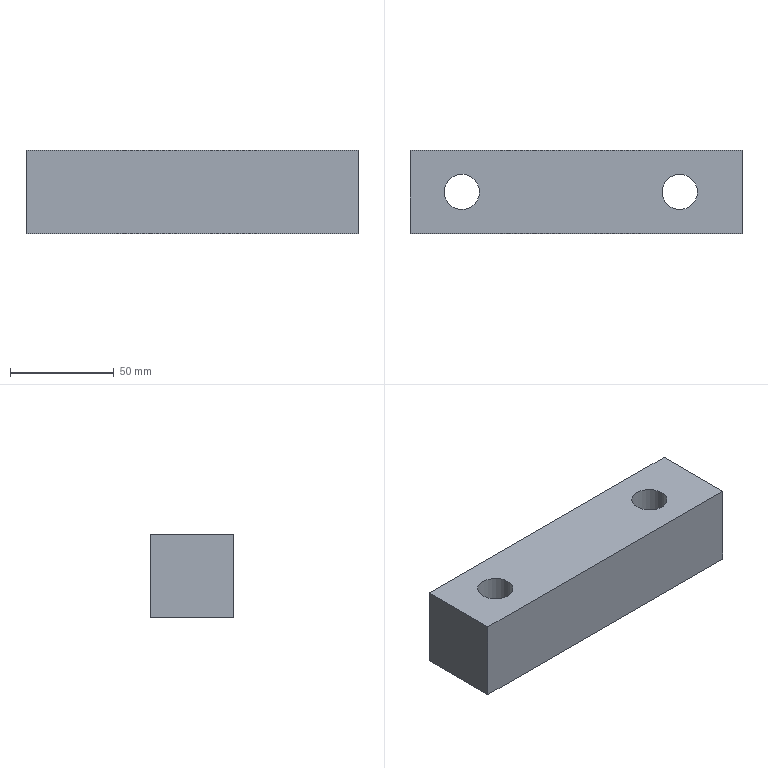Part | STEP file | 1 solid | 12 faces | box 160 x 40 x 40 mm | volume 225684 mm3 | plane 8 | cylinder 4 | commonest cylinder face diameters 17 x2 26 x2
STEP:
#1=CARTESIAN_POINT('',(87.,-262.5,-147.));
#2=VERTEX_POINT('',#1);
#3=CARTESIAN_POINT('',(100.,-262.5,-147.));
#4=DIRECTION('',(0.,0.,1.));
#5=DIRECTION('',(-1.,0.,0.));
#6=AXIS2_PLACEMENT_3D('',#3,#4,#5);
#7=CIRCLE('',#6,13.);
#8=EDGE_CURVE('',#2,#2,#7,.T.);
#9=ORIENTED_EDGE('',*,*,#8,.T.);
#10=EDGE_LOOP('',(#9));
#11=FACE_BOUND('',#10,.T.);
#12=CARTESIAN_POINT('',(218.,-262.5,-147.));
#13=VERTEX_POINT('',#12);
#14=CARTESIAN_POINT('',(205.,-262.5,-147.));
#15=DIRECTION('',(0.,0.,-1.));
#16=DIRECTION('',(1.,0.,0.));
#17=AXIS2_PLACEMENT_3D('',#14,#15,#16);
#18=CIRCLE('',#17,13.);
#19=EDGE_CURVE('',#13,#13,#18,.T.);
#20=ORIENTED_EDGE('',*,*,#19,.F.);
#21=EDGE_LOOP('',(#20));
#22=FACE_BOUND('',#21,.T.);
#23=CARTESIAN_POINT('',(235.,-282.5,-147.));
#24=VERTEX_POINT('',#23);
#25=CARTESIAN_POINT('',(75.,-282.5,-147.));
#26=VERTEX_POINT('',#25);
#27=CARTESIAN_POINT('',(65.,-282.5,-147.));
#28=DIRECTION('',(-1.,0.,0.));
#29=VECTOR('',#28,1.);
#30=LINE('',#27,#29);
#31=EDGE_CURVE('',#24,#26,#30,.T.);
#32=ORIENTED_EDGE('',*,*,#31,.T.);
#33=CARTESIAN_POINT('',(75.,-242.5,-147.));
#34=VERTEX_POINT('',#33);
#35=CARTESIAN_POINT('',(75.,-262.5,-147.));
#36=DIRECTION('',(0.,-1.,0.));
#37=VECTOR('',#36,1.);
#38=LINE('',#35,#37);
#39=EDGE_CURVE('',#34,#26,#38,.T.);
#40=ORIENTED_EDGE('',*,*,#39,.F.);
#41=CARTESIAN_POINT('',(235.,-242.5,-147.));
#42=VERTEX_POINT('',#41);
#43=CARTESIAN_POINT('',(112.5,-242.5,-147.));
#44=DIRECTION('',(-1.,0.,0.));
#45=VECTOR('',#44,1.);
#46=LINE('',#43,#45);
#47=EDGE_CURVE('',#42,#34,#46,.T.);
#48=ORIENTED_EDGE('',*,*,#47,.F.);
#49=CARTESIAN_POINT('',(235.,-243.548,-147.));
#50=DIRECTION('',(0.,-1.,0.));
#51=VECTOR('',#50,1.);
#52=LINE('',#49,#51);
#53=EDGE_CURVE('',#42,#24,#52,.T.);
#54=ORIENTED_EDGE('',*,*,#53,.T.);
#55=EDGE_LOOP('',(#32,#40,#48,#54));
#56=FACE_BOUND('',#55,.T.);
#57=CARTESIAN_POINT('',(205.,-262.5,-147.));
#58=DIRECTION('',(0.,0.,-1.));
#59=DIRECTION('',(1.,0.,0.));
#60=AXIS2_PLACEMENT_3D('',#57,#58,#59);
#61=PLANE('',#60);
#62=ADVANCED_FACE('',(#11,#22,#56),#61,.T.);
#63=CARTESIAN_POINT('',(91.5,-262.5,-107.));
#64=VERTEX_POINT('',#63);
#65=CARTESIAN_POINT('',(100.,-262.5,-107.));
#66=DIRECTION('',(0.,0.,-1.));
#67=DIRECTION('',(-1.,0.,0.));
#68=AXIS2_PLACEMENT_3D('',#65,#66,#67);
#69=CIRCLE('',#68,8.5);
#70=EDGE_CURVE('',#64,#64,#69,.T.);
#71=ORIENTED_EDGE('',*,*,#70,.T.);
#72=EDGE_LOOP('',(#71));
#73=FACE_BOUND('',#72,.T.);
#74=CARTESIAN_POINT('',(213.5,-262.5,-107.));
#75=VERTEX_POINT('',#74);
#76=CARTESIAN_POINT('',(205.,-262.5,-107.));
#77=DIRECTION('',(0.,0.,1.));
#78=DIRECTION('',(1.,0.,0.));
#79=AXIS2_PLACEMENT_3D('',#76,#77,#78);
#80=CIRCLE('',#79,8.5);
#81=EDGE_CURVE('',#75,#75,#80,.T.);
#82=ORIENTED_EDGE('',*,*,#81,.F.);
#83=EDGE_LOOP('',(#82));
#84=FACE_BOUND('',#83,.T.);
#85=CARTESIAN_POINT('',(75.,-242.5,-107.));
#86=VERTEX_POINT('',#85);
#87=CARTESIAN_POINT('',(75.,-282.5,-107.));
#88=VERTEX_POINT('',#87);
#89=CARTESIAN_POINT('',(75.,9.,-107.));
#90=DIRECTION('',(0.,-1.,0.));
#91=VECTOR('',#90,1.);
#92=LINE('',#89,#91);
#93=EDGE_CURVE('',#86,#88,#92,.T.);
#94=ORIENTED_EDGE('',*,*,#93,.T.);
#95=CARTESIAN_POINT('',(235.,-282.5,-107.));
#96=VERTEX_POINT('',#95);
#97=CARTESIAN_POINT('',(65.,-282.5,-107.));
#98=DIRECTION('',(1.,0.,0.));
#99=VECTOR('',#98,1.);
#100=LINE('',#97,#99);
#101=EDGE_CURVE('',#88,#96,#100,.T.);
#102=ORIENTED_EDGE('',*,*,#101,.T.);
#103=CARTESIAN_POINT('',(235.,-242.5,-107.));
#104=VERTEX_POINT('',#103);
#105=CARTESIAN_POINT('',(235.,9.,-107.));
#106=DIRECTION('',(0.,-1.,0.));
#107=VECTOR('',#106,1.);
#108=LINE('',#105,#107);
#109=EDGE_CURVE('',#104,#96,#108,.T.);
#110=ORIENTED_EDGE('',*,*,#109,.F.);
#111=CARTESIAN_POINT('',(65.,-242.5,-107.));
#112=DIRECTION('',(-1.,0.,0.));
#113=VECTOR('',#112,1.);
#114=LINE('',#111,#113);
#115=EDGE_CURVE('',#104,#86,#114,.T.);
#116=ORIENTED_EDGE('',*,*,#115,.T.);
#117=EDGE_LOOP('',(#94,#102,#110,#116));
#118=FACE_BOUND('',#117,.T.);
#119=CARTESIAN_POINT('',(65.,9.,-107.));
#120=DIRECTION('',(0.,0.,-1.));
#121=DIRECTION('',(0.,-1.,0.));
#122=AXIS2_PLACEMENT_3D('',#119,#120,#121);
#123=PLANE('',#122);
#124=ADVANCED_FACE('',(#73,#84,#118),#123,.F.);
#125=CARTESIAN_POINT('',(75.,-282.5,-107.));
#126=DIRECTION('',(0.,0.,1.));
#127=VECTOR('',#126,1.);
#128=LINE('',#125,#127);
#129=EDGE_CURVE('',#26,#88,#128,.T.);
#130=ORIENTED_EDGE('',*,*,#129,.T.);
#131=ORIENTED_EDGE('',*,*,#93,.F.);
#132=CARTESIAN_POINT('',(75.,-242.5,-199.5));
#133=DIRECTION('',(0.,0.,-1.));
#134=VECTOR('',#133,1.);
#135=LINE('',#132,#134);
#136=EDGE_CURVE('',#86,#34,#135,.T.);
#137=ORIENTED_EDGE('',*,*,#136,.T.);
#138=ORIENTED_EDGE('',*,*,#39,.T.);
#139=EDGE_LOOP('',(#130,#131,#137,#138));
#140=FACE_OUTER_BOUND('',#139,.T.);
#141=CARTESIAN_POINT('',(75.,9.,-107.));
#142=DIRECTION('',(1.,0.,0.));
#143=DIRECTION('',(0.,-1.,0.));
#144=AXIS2_PLACEMENT_3D('',#141,#142,#143);
#145=PLANE('',#144);
#146=ADVANCED_FACE('',(#140),#145,.F.);
#147=ORIENTED_EDGE('',*,*,#53,.F.);
#148=CARTESIAN_POINT('',(235.,-242.5,-199.5));
#149=DIRECTION('',(0.,0.,1.));
#150=VECTOR('',#149,1.);
#151=LINE('',#148,#150);
#152=EDGE_CURVE('',#42,#104,#151,.T.);
#153=ORIENTED_EDGE('',*,*,#152,.T.);
#154=ORIENTED_EDGE('',*,*,#109,.T.);
#155=CARTESIAN_POINT('',(235.,-282.5,-107.));
#156=DIRECTION('',(0.,0.,1.));
#157=VECTOR('',#156,1.);
#158=LINE('',#155,#157);
#159=EDGE_CURVE('',#24,#96,#158,.T.);
#160=ORIENTED_EDGE('',*,*,#159,.F.);
#161=EDGE_LOOP('',(#147,#153,#154,#160));
#162=FACE_OUTER_BOUND('',#161,.T.);
#163=CARTESIAN_POINT('',(235.,-243.548,-107.));
#164=DIRECTION('',(-1.,0.,0.));
#165=DIRECTION('',(0.,0.,1.));
#166=AXIS2_PLACEMENT_3D('',#163,#164,#165);
#167=PLANE('',#166);
#168=ADVANCED_FACE('',(#162),#167,.F.);
#169=ORIENTED_EDGE('',*,*,#159,.T.);
#170=ORIENTED_EDGE('',*,*,#101,.F.);
#171=ORIENTED_EDGE('',*,*,#129,.F.);
#172=ORIENTED_EDGE('',*,*,#31,.F.);
#173=EDGE_LOOP('',(#169,#170,#171,#172));
#174=FACE_OUTER_BOUND('',#173,.T.);
#175=CARTESIAN_POINT('',(65.,-282.5,-107.));
#176=DIRECTION('',(0.,1.,0.));
#177=DIRECTION('',(0.,0.,-1.));
#178=AXIS2_PLACEMENT_3D('',#175,#176,#177);
#179=PLANE('',#178);
#180=ADVANCED_FACE('',(#174),#179,.F.);
#181=ORIENTED_EDGE('',*,*,#136,.F.);
#182=ORIENTED_EDGE('',*,*,#115,.F.);
#183=ORIENTED_EDGE('',*,*,#152,.F.);
#184=ORIENTED_EDGE('',*,*,#47,.T.);
#185=EDGE_LOOP('',(#181,#182,#183,#184));
#186=FACE_OUTER_BOUND('',#185,.T.);
#187=CARTESIAN_POINT('',(112.5,-242.5,-199.5));
#188=DIRECTION('',(0.,1.,0.));
#189=DIRECTION('',(0.,0.,1.));
#190=AXIS2_PLACEMENT_3D('',#187,#188,#189);
#191=PLANE('',#190);
#192=ADVANCED_FACE('',(#186),#191,.T.);
#193=CARTESIAN_POINT('',(196.5,-262.5,-127.));
#194=VERTEX_POINT('',#193);
#195=CARTESIAN_POINT('',(205.,-262.5,-127.));
#196=DIRECTION('',(0.,0.,-1.));
#197=DIRECTION('',(-1.,0.,0.));
#198=AXIS2_PLACEMENT_3D('',#195,#196,#197);
#199=CIRCLE('',#198,8.5);
#200=EDGE_CURVE('',#194,#194,#199,.T.);
#201=ORIENTED_EDGE('',*,*,#200,.T.);
#202=EDGE_LOOP('',(#201));
#203=FACE_BOUND('',#202,.T.);
#204=ORIENTED_EDGE('',*,*,#81,.T.);
#205=EDGE_LOOP('',(#204));
#206=FACE_BOUND('',#205,.T.);
#207=CARTESIAN_POINT('',(205.,-262.5,-107.));
#208=DIRECTION('',(0.,0.,-1.));
#209=DIRECTION('',(1.,0.,0.));
#210=AXIS2_PLACEMENT_3D('',#207,#208,#209);
#211=CYLINDRICAL_SURFACE('',#210,8.5);
#212=ADVANCED_FACE('',(#203,#206),#211,.F.);
#213=ORIENTED_EDGE('',*,*,#200,.F.);
#214=EDGE_LOOP('',(#213));
#215=FACE_BOUND('',#214,.T.);
#216=CARTESIAN_POINT('',(218.,-262.5,-127.));
#217=VERTEX_POINT('',#216);
#218=CARTESIAN_POINT('',(205.,-262.5,-127.));
#219=DIRECTION('',(0.,0.,-1.));
#220=DIRECTION('',(1.,0.,0.));
#221=AXIS2_PLACEMENT_3D('',#218,#219,#220);
#222=CIRCLE('',#221,13.);
#223=EDGE_CURVE('',#217,#217,#222,.T.);
#224=ORIENTED_EDGE('',*,*,#223,.T.);
#225=EDGE_LOOP('',(#224));
#226=FACE_BOUND('',#225,.T.);
#227=CARTESIAN_POINT('',(205.,-262.5,-127.));
#228=DIRECTION('',(0.,0.,1.));
#229=DIRECTION('',(-1.,0.,0.));
#230=AXIS2_PLACEMENT_3D('',#227,#228,#229);
#231=PLANE('',#230);
#232=ADVANCED_FACE('',(#215,#226),#231,.F.);
#233=ORIENTED_EDGE('',*,*,#19,.T.);
#234=EDGE_LOOP('',(#233));
#235=FACE_BOUND('',#234,.T.);
#236=ORIENTED_EDGE('',*,*,#223,.F.);
#237=EDGE_LOOP('',(#236));
#238=FACE_BOUND('',#237,.T.);
#239=CARTESIAN_POINT('',(205.,-262.5,-127.));
#240=DIRECTION('',(0.,0.,-1.));
#241=DIRECTION('',(1.,0.,0.));
#242=AXIS2_PLACEMENT_3D('',#239,#240,#241);
#243=CYLINDRICAL_SURFACE('',#242,13.);
#244=ADVANCED_FACE('',(#235,#238),#243,.F.);
#245=CARTESIAN_POINT('',(108.5,-262.5,-127.));
#246=VERTEX_POINT('',#245);
#247=CARTESIAN_POINT('',(100.,-262.5,-127.));
#248=DIRECTION('',(0.,0.,1.));
#249=DIRECTION('',(1.,0.,0.));
#250=AXIS2_PLACEMENT_3D('',#247,#248,#249);
#251=CIRCLE('',#250,8.5);
#252=EDGE_CURVE('',#246,#246,#251,.T.);
#253=ORIENTED_EDGE('',*,*,#252,.F.);
#254=EDGE_LOOP('',(#253));
#255=FACE_BOUND('',#254,.T.);
#256=ORIENTED_EDGE('',*,*,#70,.F.);
#257=EDGE_LOOP('',(#256));
#258=FACE_BOUND('',#257,.T.);
#259=CARTESIAN_POINT('',(100.,-262.5,-107.));
#260=DIRECTION('',(0.,0.,-1.));
#261=DIRECTION('',(-1.,0.,0.));
#262=AXIS2_PLACEMENT_3D('',#259,#260,#261);
#263=CYLINDRICAL_SURFACE('',#262,8.5);
#264=ADVANCED_FACE('',(#255,#258),#263,.F.);
#265=ORIENTED_EDGE('',*,*,#252,.T.);
#266=EDGE_LOOP('',(#265));
#267=FACE_BOUND('',#266,.T.);
#268=CARTESIAN_POINT('',(87.,-262.5,-127.));
#269=VERTEX_POINT('',#268);
#270=CARTESIAN_POINT('',(100.,-262.5,-127.));
#271=DIRECTION('',(0.,0.,1.));
#272=DIRECTION('',(-1.,0.,0.));
#273=AXIS2_PLACEMENT_3D('',#270,#271,#272);
#274=CIRCLE('',#273,13.);
#275=EDGE_CURVE('',#269,#269,#274,.T.);
#276=ORIENTED_EDGE('',*,*,#275,.F.);
#277=EDGE_LOOP('',(#276));
#278=FACE_BOUND('',#277,.T.);
#279=CARTESIAN_POINT('',(100.,-262.5,-127.));
#280=DIRECTION('',(0.,0.,1.));
#281=DIRECTION('',(1.,0.,0.));
#282=AXIS2_PLACEMENT_3D('',#279,#280,#281);
#283=PLANE('',#282);
#284=ADVANCED_FACE('',(#267,#278),#283,.F.);
#285=ORIENTED_EDGE('',*,*,#8,.F.);
#286=EDGE_LOOP('',(#285));
#287=FACE_BOUND('',#286,.T.);
#288=ORIENTED_EDGE('',*,*,#275,.T.);
#289=EDGE_LOOP('',(#288));
#290=FACE_BOUND('',#289,.T.);
#291=CARTESIAN_POINT('',(100.,-262.5,-127.));
#292=DIRECTION('',(0.,0.,-1.));
#293=DIRECTION('',(-1.,0.,0.));
#294=AXIS2_PLACEMENT_3D('',#291,#292,#293);
#295=CYLINDRICAL_SURFACE('',#294,13.);
#296=ADVANCED_FACE('',(#287,#290),#295,.F.);
#297=CLOSED_SHELL('',(#62,#124,#146,#168,#180,#192,#212,#232,#244,#264,#284,#296));
#298=MANIFOLD_SOLID_BREP('',#297);
#299=(LENGTH_UNIT()NAMED_UNIT(*)SI_UNIT(.MILLI.,.METRE.));
#300=UNCERTAINTY_MEASURE_WITH_UNIT(LENGTH_MEASURE(0.00002),#299,'','');
#301=(NAMED_UNIT(*)PLANE_ANGLE_UNIT()SI_UNIT($,.RADIAN.));
#302=PLANE_ANGLE_MEASURE_WITH_UNIT(PLANE_ANGLE_MEASURE(0.01745),#301);
#303=DIMENSIONAL_EXPONENTS(0.,0.,0.,0.,0.,0.,0.);
#304=(CONVERSION_BASED_UNIT('DEGREE',#302)NAMED_UNIT(#303)PLANE_ANGLE_UNIT());
#305=(NAMED_UNIT(*)SI_UNIT($,.STERADIAN.)SOLID_ANGLE_UNIT());
#306=(GEOMETRIC_REPRESENTATION_CONTEXT(3)GLOBAL_UNCERTAINTY_ASSIGNED_CONTEXT((#300))GLOBAL_UNIT_ASSIGNED_CONTEXT((#299,#304,#305))REPRESENTATION_CONTEXT('',''));
#307=ADVANCED_BREP_SHAPE_REPRESENTATION('',(#298),#306);